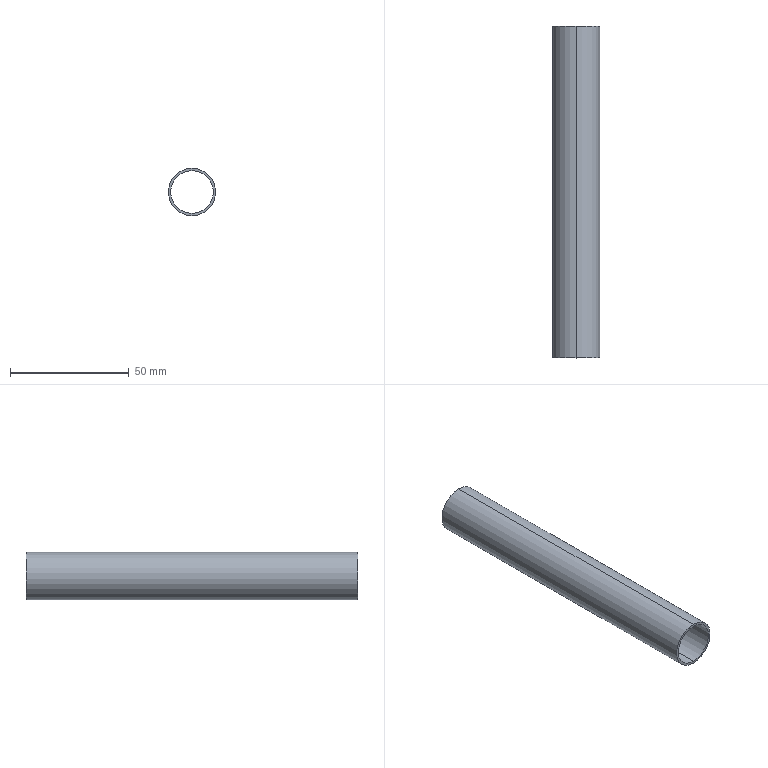Part | SolidWorks | features Extrusion 1 | 1 solid | 6 faces | box 20 x 140 x 20 mm | volume 8357 mm3 | cylinder 4 | plane 2 | commonest cylinder face diameters 18 x2 20 x2
STEP:
#1=CARTESIAN_POINT('',(0.,140.,-9.));
#2=VERTEX_POINT('',#1);
#3=CARTESIAN_POINT('',(0.,140.,9.));
#4=VERTEX_POINT('',#3);
#5=CARTESIAN_POINT('',(0.,140.,0.));
#6=DIRECTION('',(0.,1.,0.));
#7=DIRECTION('',(0.,0.,1.));
#8=AXIS2_PLACEMENT_3D('',#5,#6,#7);
#9=CIRCLE('',#8,9.);
#10=EDGE_CURVE('',#2,#4,#9,.T.);
#11=ORIENTED_EDGE('',*,*,#10,.T.);
#12=CARTESIAN_POINT('',(0.,0.,9.));
#13=VERTEX_POINT('',#12);
#14=CARTESIAN_POINT('',(0.,140.,9.));
#15=DIRECTION('',(0.,-1.,0.));
#16=VECTOR('',#15,1000.);
#17=LINE('',#14,#16);
#18=EDGE_CURVE('',#4,#13,#17,.T.);
#19=ORIENTED_EDGE('',*,*,#18,.T.);
#20=CARTESIAN_POINT('',(0.,0.,-9.));
#21=VERTEX_POINT('',#20);
#22=CARTESIAN_POINT('',(0.,0.,0.));
#23=DIRECTION('',(0.,1.,0.));
#24=DIRECTION('',(0.,0.,1.));
#25=AXIS2_PLACEMENT_3D('',#22,#23,#24);
#26=CIRCLE('',#25,9.);
#27=EDGE_CURVE('',#21,#13,#26,.T.);
#28=ORIENTED_EDGE('',*,*,#27,.F.);
#29=CARTESIAN_POINT('',(0.,140.,-9.));
#30=DIRECTION('',(0.,-1.,0.));
#31=VECTOR('',#30,1000.);
#32=LINE('',#29,#31);
#33=EDGE_CURVE('',#2,#21,#32,.T.);
#34=ORIENTED_EDGE('',*,*,#33,.F.);
#35=EDGE_LOOP('',(#11,#19,#28,#34));
#36=FACE_OUTER_BOUND('',#35,.T.);
#37=CARTESIAN_POINT('',(0.,140.,0.));
#38=DIRECTION('',(0.,-1.,0.));
#39=DIRECTION('',(0.,0.,-1.));
#40=AXIS2_PLACEMENT_3D('',#37,#38,#39);
#41=CYLINDRICAL_SURFACE('',#40,9.);
#42=ADVANCED_FACE('',(#36),#41,.F.);
#43=CARTESIAN_POINT('',(0.,140.,10.));
#44=VERTEX_POINT('',#43);
#45=CARTESIAN_POINT('',(0.,140.,-10.));
#46=VERTEX_POINT('',#45);
#47=CARTESIAN_POINT('',(0.,140.,0.));
#48=DIRECTION('',(0.,1.,0.));
#49=DIRECTION('',(0.,0.,1.));
#50=AXIS2_PLACEMENT_3D('',#47,#48,#49);
#51=CIRCLE('',#50,10.);
#52=EDGE_CURVE('',#44,#46,#51,.T.);
#53=ORIENTED_EDGE('',*,*,#52,.F.);
#54=CARTESIAN_POINT('',(0.,0.,10.));
#55=VERTEX_POINT('',#54);
#56=CARTESIAN_POINT('',(0.,140.,10.));
#57=DIRECTION('',(0.,-1.,0.));
#58=VECTOR('',#57,1000.);
#59=LINE('',#56,#58);
#60=EDGE_CURVE('',#44,#55,#59,.T.);
#61=ORIENTED_EDGE('',*,*,#60,.T.);
#62=CARTESIAN_POINT('',(0.,0.,-10.));
#63=VERTEX_POINT('',#62);
#64=CARTESIAN_POINT('',(0.,0.,0.));
#65=DIRECTION('',(0.,1.,0.));
#66=DIRECTION('',(0.,0.,1.));
#67=AXIS2_PLACEMENT_3D('',#64,#65,#66);
#68=CIRCLE('',#67,10.);
#69=EDGE_CURVE('',#55,#63,#68,.T.);
#70=ORIENTED_EDGE('',*,*,#69,.T.);
#71=CARTESIAN_POINT('',(0.,140.,-10.));
#72=DIRECTION('',(0.,-1.,0.));
#73=VECTOR('',#72,1000.);
#74=LINE('',#71,#73);
#75=EDGE_CURVE('',#46,#63,#74,.T.);
#76=ORIENTED_EDGE('',*,*,#75,.F.);
#77=EDGE_LOOP('',(#53,#61,#70,#76));
#78=FACE_OUTER_BOUND('',#77,.T.);
#79=CARTESIAN_POINT('',(0.,140.,0.));
#80=DIRECTION('',(0.,-1.,0.));
#81=DIRECTION('',(0.,0.,-1.));
#82=AXIS2_PLACEMENT_3D('',#79,#80,#81);
#83=CYLINDRICAL_SURFACE('',#82,10.);
#84=ADVANCED_FACE('',(#78),#83,.T.);
#85=CARTESIAN_POINT('',(0.,140.,0.));
#86=DIRECTION('',(0.,1.,0.));
#87=DIRECTION('',(0.,0.,1.));
#88=AXIS2_PLACEMENT_3D('',#85,#86,#87);
#89=CIRCLE('',#88,10.);
#90=EDGE_CURVE('',#46,#44,#89,.T.);
#91=ORIENTED_EDGE('',*,*,#90,.T.);
#92=ORIENTED_EDGE('',*,*,#52,.T.);
#93=EDGE_LOOP('',(#91,#92));
#94=FACE_OUTER_BOUND('',#93,.T.);
#95=ORIENTED_EDGE('',*,*,#10,.F.);
#96=CARTESIAN_POINT('',(0.,140.,0.));
#97=DIRECTION('',(0.,1.,0.));
#98=DIRECTION('',(0.,0.,1.));
#99=AXIS2_PLACEMENT_3D('',#96,#97,#98);
#100=CIRCLE('',#99,9.);
#101=EDGE_CURVE('',#4,#2,#100,.T.);
#102=ORIENTED_EDGE('',*,*,#101,.F.);
#103=EDGE_LOOP('',(#95,#102));
#104=FACE_BOUND('',#103,.T.);
#105=CARTESIAN_POINT('',(0.,140.,0.));
#106=DIRECTION('',(0.,1.,0.));
#107=DIRECTION('',(0.,0.,1.));
#108=AXIS2_PLACEMENT_3D('',#105,#106,#107);
#109=PLANE('',#108);
#110=ADVANCED_FACE('',(#94,#104),#109,.T.);
#111=CARTESIAN_POINT('',(0.,0.,0.));
#112=DIRECTION('',(0.,1.,0.));
#113=DIRECTION('',(0.,0.,1.));
#114=AXIS2_PLACEMENT_3D('',#111,#112,#113);
#115=CIRCLE('',#114,10.);
#116=EDGE_CURVE('',#63,#55,#115,.T.);
#117=ORIENTED_EDGE('',*,*,#116,.F.);
#118=ORIENTED_EDGE('',*,*,#69,.F.);
#119=EDGE_LOOP('',(#117,#118));
#120=FACE_OUTER_BOUND('',#119,.T.);
#121=ORIENTED_EDGE('',*,*,#27,.T.);
#122=CARTESIAN_POINT('',(0.,0.,0.));
#123=DIRECTION('',(0.,1.,0.));
#124=DIRECTION('',(0.,0.,1.));
#125=AXIS2_PLACEMENT_3D('',#122,#123,#124);
#126=CIRCLE('',#125,9.);
#127=EDGE_CURVE('',#13,#21,#126,.T.);
#128=ORIENTED_EDGE('',*,*,#127,.T.);
#129=EDGE_LOOP('',(#121,#128));
#130=FACE_BOUND('',#129,.T.);
#131=CARTESIAN_POINT('',(0.,0.,0.));
#132=DIRECTION('',(0.,1.,0.));
#133=DIRECTION('',(0.,0.,1.));
#134=AXIS2_PLACEMENT_3D('',#131,#132,#133);
#135=PLANE('',#134);
#136=ADVANCED_FACE('',(#120,#130),#135,.F.);
#137=ORIENTED_EDGE('',*,*,#60,.F.);
#138=ORIENTED_EDGE('',*,*,#90,.F.);
#139=ORIENTED_EDGE('',*,*,#75,.T.);
#140=ORIENTED_EDGE('',*,*,#116,.T.);
#141=EDGE_LOOP('',(#137,#138,#139,#140));
#142=FACE_OUTER_BOUND('',#141,.T.);
#143=CARTESIAN_POINT('',(0.,140.,0.));
#144=DIRECTION('',(0.,-1.,0.));
#145=DIRECTION('',(0.,0.,-1.));
#146=AXIS2_PLACEMENT_3D('',#143,#144,#145);
#147=CYLINDRICAL_SURFACE('',#146,10.);
#148=ADVANCED_FACE('',(#142),#147,.T.);
#149=ORIENTED_EDGE('',*,*,#18,.F.);
#150=ORIENTED_EDGE('',*,*,#101,.T.);
#151=ORIENTED_EDGE('',*,*,#33,.T.);
#152=ORIENTED_EDGE('',*,*,#127,.F.);
#153=EDGE_LOOP('',(#149,#150,#151,#152));
#154=FACE_OUTER_BOUND('',#153,.T.);
#155=CARTESIAN_POINT('',(0.,140.,0.));
#156=DIRECTION('',(0.,-1.,0.));
#157=DIRECTION('',(0.,0.,-1.));
#158=AXIS2_PLACEMENT_3D('',#155,#156,#157);
#159=CYLINDRICAL_SURFACE('',#158,9.);
#160=ADVANCED_FACE('',(#154),#159,.F.);
#161=CLOSED_SHELL('',(#42,#84,#110,#136,#148,#160));
#162=MANIFOLD_SOLID_BREP('',#161);
#163=CARTESIAN_POINT('',(0.,0.,0.));
#164=DIRECTION('',(0.,0.,1.));
#165=DIRECTION('',(1.,0.,0.));
#166=AXIS2_PLACEMENT_3D('',#163,#164,#165);
#167=(LENGTH_UNIT()NAMED_UNIT(*)SI_UNIT(.MILLI.,.METRE.));
#168=UNCERTAINTY_MEASURE_WITH_UNIT(LENGTH_MEASURE(0.00001),#167,'','');
#169=(NAMED_UNIT(*)PLANE_ANGLE_UNIT()SI_UNIT($,.RADIAN.));
#170=(NAMED_UNIT(*)SI_UNIT($,.STERADIAN.)SOLID_ANGLE_UNIT());
#171=(GEOMETRIC_REPRESENTATION_CONTEXT(3)GLOBAL_UNCERTAINTY_ASSIGNED_CONTEXT((#168))GLOBAL_UNIT_ASSIGNED_CONTEXT((#167,#169,#170))REPRESENTATION_CONTEXT('',''));
#172=ADVANCED_BREP_SHAPE_REPRESENTATION('',(#162,#166),#171);